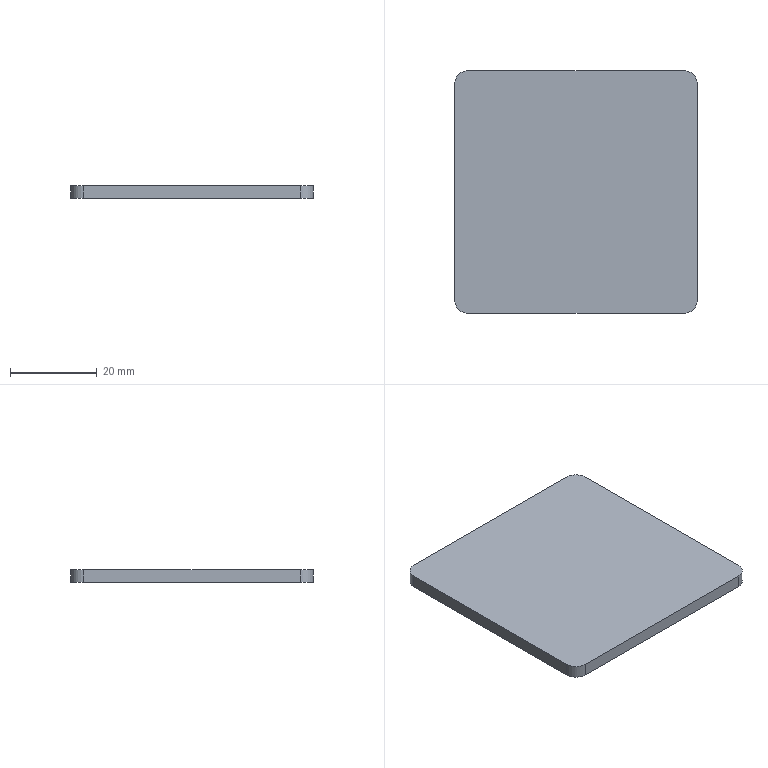Part | STEP file | 750038152 | 1 solid | 10 faces | box 56 x 56 x 3 mm | volume 9385 mm3 | plane 6 | cylinder 4 | commonest cylinder face diameters 6 x4
STEP:
#1=CARTESIAN_POINT('',(28.,25.,3.));
#2=VERTEX_POINT('',#1);
#3=CARTESIAN_POINT('',(25.,28.,3.));
#4=VERTEX_POINT('',#3);
#5=CARTESIAN_POINT('',(25.,25.,3.));
#6=DIRECTION('',(0.,0.,1.));
#7=DIRECTION('',(-1.,0.,0.));
#8=AXIS2_PLACEMENT_3D('',#5,#6,#7);
#9=CIRCLE('',#8,3.);
#10=EDGE_CURVE('',#2,#4,#9,.T.);
#11=ORIENTED_EDGE('',*,*,#10,.T.);
#12=CARTESIAN_POINT('',(-25.,28.,3.));
#13=VERTEX_POINT('',#12);
#14=CARTESIAN_POINT('',(-25.,28.,3.));
#15=DIRECTION('',(-1.,0.,0.));
#16=VECTOR('',#15,1000.);
#17=LINE('',#14,#16);
#18=EDGE_CURVE('',#4,#13,#17,.T.);
#19=ORIENTED_EDGE('',*,*,#18,.T.);
#20=CARTESIAN_POINT('',(-28.,25.,3.));
#21=VERTEX_POINT('',#20);
#22=CARTESIAN_POINT('',(-25.,25.,3.));
#23=DIRECTION('',(0.,0.,1.));
#24=DIRECTION('',(-1.,0.,0.));
#25=AXIS2_PLACEMENT_3D('',#22,#23,#24);
#26=CIRCLE('',#25,3.);
#27=EDGE_CURVE('',#13,#21,#26,.T.);
#28=ORIENTED_EDGE('',*,*,#27,.T.);
#29=CARTESIAN_POINT('',(-28.,-25.,3.));
#30=VERTEX_POINT('',#29);
#31=CARTESIAN_POINT('',(-28.,25.,3.));
#32=DIRECTION('',(0.,-1.,0.));
#33=VECTOR('',#32,1000.);
#34=LINE('',#31,#33);
#35=EDGE_CURVE('',#21,#30,#34,.T.);
#36=ORIENTED_EDGE('',*,*,#35,.T.);
#37=CARTESIAN_POINT('',(-25.,-28.,3.));
#38=VERTEX_POINT('',#37);
#39=CARTESIAN_POINT('',(-25.,-25.,3.));
#40=DIRECTION('',(0.,0.,1.));
#41=DIRECTION('',(-1.,0.,0.));
#42=AXIS2_PLACEMENT_3D('',#39,#40,#41);
#43=CIRCLE('',#42,3.);
#44=EDGE_CURVE('',#30,#38,#43,.T.);
#45=ORIENTED_EDGE('',*,*,#44,.T.);
#46=CARTESIAN_POINT('',(25.,-28.,3.));
#47=VERTEX_POINT('',#46);
#48=CARTESIAN_POINT('',(-25.,-28.,3.));
#49=DIRECTION('',(1.,0.,0.));
#50=VECTOR('',#49,1000.);
#51=LINE('',#48,#50);
#52=EDGE_CURVE('',#38,#47,#51,.T.);
#53=ORIENTED_EDGE('',*,*,#52,.T.);
#54=CARTESIAN_POINT('',(28.,-25.,3.));
#55=VERTEX_POINT('',#54);
#56=CARTESIAN_POINT('',(25.,-25.,3.));
#57=DIRECTION('',(0.,0.,1.));
#58=DIRECTION('',(-1.,0.,0.));
#59=AXIS2_PLACEMENT_3D('',#56,#57,#58);
#60=CIRCLE('',#59,3.);
#61=EDGE_CURVE('',#47,#55,#60,.T.);
#62=ORIENTED_EDGE('',*,*,#61,.T.);
#63=CARTESIAN_POINT('',(28.,25.,3.));
#64=DIRECTION('',(0.,1.,0.));
#65=VECTOR('',#64,1000.);
#66=LINE('',#63,#65);
#67=EDGE_CURVE('',#55,#2,#66,.T.);
#68=ORIENTED_EDGE('',*,*,#67,.T.);
#69=EDGE_LOOP('',(#11,#19,#28,#36,#45,#53,#62,#68));
#70=FACE_OUTER_BOUND('',#69,.T.);
#71=CARTESIAN_POINT('',(-25.,25.,3.));
#72=DIRECTION('',(0.,0.,1.));
#73=DIRECTION('',(1.,0.,0.));
#74=AXIS2_PLACEMENT_3D('',#71,#72,#73);
#75=PLANE('',#74);
#76=ADVANCED_FACE('',(#70),#75,.T.);
#77=CARTESIAN_POINT('',(-25.,28.,0.));
#78=VERTEX_POINT('',#77);
#79=CARTESIAN_POINT('',(-25.,28.,3.));
#80=DIRECTION('',(0.,0.,-1.));
#81=VECTOR('',#80,1000.);
#82=LINE('',#79,#81);
#83=EDGE_CURVE('',#13,#78,#82,.T.);
#84=ORIENTED_EDGE('',*,*,#83,.F.);
#85=ORIENTED_EDGE('',*,*,#18,.F.);
#86=CARTESIAN_POINT('',(25.,28.,0.));
#87=VERTEX_POINT('',#86);
#88=CARTESIAN_POINT('',(25.,28.,3.));
#89=DIRECTION('',(0.,0.,1.));
#90=VECTOR('',#89,1000.);
#91=LINE('',#88,#90);
#92=EDGE_CURVE('',#87,#4,#91,.T.);
#93=ORIENTED_EDGE('',*,*,#92,.F.);
#94=CARTESIAN_POINT('',(25.,28.,0.));
#95=DIRECTION('',(1.,0.,0.));
#96=VECTOR('',#95,1000.);
#97=LINE('',#94,#96);
#98=EDGE_CURVE('',#78,#87,#97,.T.);
#99=ORIENTED_EDGE('',*,*,#98,.F.);
#100=EDGE_LOOP('',(#84,#85,#93,#99));
#101=FACE_OUTER_BOUND('',#100,.T.);
#102=CARTESIAN_POINT('',(25.,28.,3.));
#103=DIRECTION('',(0.,-1.,0.));
#104=DIRECTION('',(0.,0.,-1.));
#105=AXIS2_PLACEMENT_3D('',#102,#103,#104);
#106=PLANE('',#105);
#107=ADVANCED_FACE('',(#101),#106,.F.);
#108=ORIENTED_EDGE('',*,*,#10,.F.);
#109=CARTESIAN_POINT('',(28.,25.,0.));
#110=VERTEX_POINT('',#109);
#111=CARTESIAN_POINT('',(28.,25.,3.));
#112=DIRECTION('',(0.,0.,-1.));
#113=VECTOR('',#112,1000.);
#114=LINE('',#111,#113);
#115=EDGE_CURVE('',#2,#110,#114,.T.);
#116=ORIENTED_EDGE('',*,*,#115,.T.);
#117=CARTESIAN_POINT('',(25.,25.,0.));
#118=DIRECTION('',(0.,0.,1.));
#119=DIRECTION('',(-1.,0.,0.));
#120=AXIS2_PLACEMENT_3D('',#117,#118,#119);
#121=CIRCLE('',#120,3.);
#122=EDGE_CURVE('',#110,#87,#121,.T.);
#123=ORIENTED_EDGE('',*,*,#122,.T.);
#124=ORIENTED_EDGE('',*,*,#92,.T.);
#125=EDGE_LOOP('',(#108,#116,#123,#124));
#126=FACE_OUTER_BOUND('',#125,.T.);
#127=CARTESIAN_POINT('',(25.,25.,3.));
#128=DIRECTION('',(0.,0.,-1.));
#129=DIRECTION('',(-1.,0.,0.));
#130=AXIS2_PLACEMENT_3D('',#127,#128,#129);
#131=CYLINDRICAL_SURFACE('',#130,3.);
#132=ADVANCED_FACE('',(#126),#131,.T.);
#133=ORIENTED_EDGE('',*,*,#115,.F.);
#134=ORIENTED_EDGE('',*,*,#67,.F.);
#135=CARTESIAN_POINT('',(28.,-25.,0.));
#136=VERTEX_POINT('',#135);
#137=CARTESIAN_POINT('',(28.,-25.,3.));
#138=DIRECTION('',(0.,0.,1.));
#139=VECTOR('',#138,1000.);
#140=LINE('',#137,#139);
#141=EDGE_CURVE('',#136,#55,#140,.T.);
#142=ORIENTED_EDGE('',*,*,#141,.F.);
#143=CARTESIAN_POINT('',(28.,-25.,0.));
#144=DIRECTION('',(0.,-1.,0.));
#145=VECTOR('',#144,1000.);
#146=LINE('',#143,#145);
#147=EDGE_CURVE('',#110,#136,#146,.T.);
#148=ORIENTED_EDGE('',*,*,#147,.F.);
#149=EDGE_LOOP('',(#133,#134,#142,#148));
#150=FACE_OUTER_BOUND('',#149,.T.);
#151=CARTESIAN_POINT('',(28.,-25.,3.));
#152=DIRECTION('',(-1.,0.,0.));
#153=DIRECTION('',(0.,-1.,0.));
#154=AXIS2_PLACEMENT_3D('',#151,#152,#153);
#155=PLANE('',#154);
#156=ADVANCED_FACE('',(#150),#155,.F.);
#157=ORIENTED_EDGE('',*,*,#61,.F.);
#158=CARTESIAN_POINT('',(25.,-28.,0.));
#159=VERTEX_POINT('',#158);
#160=CARTESIAN_POINT('',(25.,-28.,3.));
#161=DIRECTION('',(0.,0.,-1.));
#162=VECTOR('',#161,1000.);
#163=LINE('',#160,#162);
#164=EDGE_CURVE('',#47,#159,#163,.T.);
#165=ORIENTED_EDGE('',*,*,#164,.T.);
#166=CARTESIAN_POINT('',(25.,-25.,0.));
#167=DIRECTION('',(0.,0.,1.));
#168=DIRECTION('',(-1.,0.,0.));
#169=AXIS2_PLACEMENT_3D('',#166,#167,#168);
#170=CIRCLE('',#169,3.);
#171=EDGE_CURVE('',#159,#136,#170,.T.);
#172=ORIENTED_EDGE('',*,*,#171,.T.);
#173=ORIENTED_EDGE('',*,*,#141,.T.);
#174=EDGE_LOOP('',(#157,#165,#172,#173));
#175=FACE_OUTER_BOUND('',#174,.T.);
#176=CARTESIAN_POINT('',(25.,-25.,3.));
#177=DIRECTION('',(0.,0.,-1.));
#178=DIRECTION('',(-1.,0.,0.));
#179=AXIS2_PLACEMENT_3D('',#176,#177,#178);
#180=CYLINDRICAL_SURFACE('',#179,3.);
#181=ADVANCED_FACE('',(#175),#180,.T.);
#182=ORIENTED_EDGE('',*,*,#164,.F.);
#183=ORIENTED_EDGE('',*,*,#52,.F.);
#184=CARTESIAN_POINT('',(-25.,-28.,0.));
#185=VERTEX_POINT('',#184);
#186=CARTESIAN_POINT('',(-25.,-28.,3.));
#187=DIRECTION('',(0.,0.,1.));
#188=VECTOR('',#187,1000.);
#189=LINE('',#186,#188);
#190=EDGE_CURVE('',#185,#38,#189,.T.);
#191=ORIENTED_EDGE('',*,*,#190,.F.);
#192=CARTESIAN_POINT('',(-25.,-28.,0.));
#193=DIRECTION('',(-1.,0.,0.));
#194=VECTOR('',#193,1000.);
#195=LINE('',#192,#194);
#196=EDGE_CURVE('',#159,#185,#195,.T.);
#197=ORIENTED_EDGE('',*,*,#196,.F.);
#198=EDGE_LOOP('',(#182,#183,#191,#197));
#199=FACE_OUTER_BOUND('',#198,.T.);
#200=CARTESIAN_POINT('',(-25.,-28.,3.));
#201=DIRECTION('',(0.,1.,0.));
#202=DIRECTION('',(0.,0.,1.));
#203=AXIS2_PLACEMENT_3D('',#200,#201,#202);
#204=PLANE('',#203);
#205=ADVANCED_FACE('',(#199),#204,.F.);
#206=ORIENTED_EDGE('',*,*,#44,.F.);
#207=CARTESIAN_POINT('',(-28.,-25.,0.));
#208=VERTEX_POINT('',#207);
#209=CARTESIAN_POINT('',(-28.,-25.,3.));
#210=DIRECTION('',(0.,0.,-1.));
#211=VECTOR('',#210,1000.);
#212=LINE('',#209,#211);
#213=EDGE_CURVE('',#30,#208,#212,.T.);
#214=ORIENTED_EDGE('',*,*,#213,.T.);
#215=CARTESIAN_POINT('',(-25.,-25.,0.));
#216=DIRECTION('',(0.,0.,1.));
#217=DIRECTION('',(-1.,0.,0.));
#218=AXIS2_PLACEMENT_3D('',#215,#216,#217);
#219=CIRCLE('',#218,3.);
#220=EDGE_CURVE('',#208,#185,#219,.T.);
#221=ORIENTED_EDGE('',*,*,#220,.T.);
#222=ORIENTED_EDGE('',*,*,#190,.T.);
#223=EDGE_LOOP('',(#206,#214,#221,#222));
#224=FACE_OUTER_BOUND('',#223,.T.);
#225=CARTESIAN_POINT('',(-25.,-25.,3.));
#226=DIRECTION('',(0.,0.,-1.));
#227=DIRECTION('',(-1.,0.,0.));
#228=AXIS2_PLACEMENT_3D('',#225,#226,#227);
#229=CYLINDRICAL_SURFACE('',#228,3.);
#230=ADVANCED_FACE('',(#224),#229,.T.);
#231=ORIENTED_EDGE('',*,*,#213,.F.);
#232=ORIENTED_EDGE('',*,*,#35,.F.);
#233=CARTESIAN_POINT('',(-28.,25.,0.));
#234=VERTEX_POINT('',#233);
#235=CARTESIAN_POINT('',(-28.,25.,3.));
#236=DIRECTION('',(0.,0.,1.));
#237=VECTOR('',#236,1000.);
#238=LINE('',#235,#237);
#239=EDGE_CURVE('',#234,#21,#238,.T.);
#240=ORIENTED_EDGE('',*,*,#239,.F.);
#241=CARTESIAN_POINT('',(-28.,25.,0.));
#242=DIRECTION('',(0.,1.,0.));
#243=VECTOR('',#242,1000.);
#244=LINE('',#241,#243);
#245=EDGE_CURVE('',#208,#234,#244,.T.);
#246=ORIENTED_EDGE('',*,*,#245,.F.);
#247=EDGE_LOOP('',(#231,#232,#240,#246));
#248=FACE_OUTER_BOUND('',#247,.T.);
#249=CARTESIAN_POINT('',(-28.,25.,3.));
#250=DIRECTION('',(1.,0.,0.));
#251=DIRECTION('',(0.,1.,0.));
#252=AXIS2_PLACEMENT_3D('',#249,#250,#251);
#253=PLANE('',#252);
#254=ADVANCED_FACE('',(#248),#253,.F.);
#255=ORIENTED_EDGE('',*,*,#27,.F.);
#256=ORIENTED_EDGE('',*,*,#83,.T.);
#257=CARTESIAN_POINT('',(-25.,25.,0.));
#258=DIRECTION('',(0.,0.,1.));
#259=DIRECTION('',(-1.,0.,0.));
#260=AXIS2_PLACEMENT_3D('',#257,#258,#259);
#261=CIRCLE('',#260,3.);
#262=EDGE_CURVE('',#78,#234,#261,.T.);
#263=ORIENTED_EDGE('',*,*,#262,.T.);
#264=ORIENTED_EDGE('',*,*,#239,.T.);
#265=EDGE_LOOP('',(#255,#256,#263,#264));
#266=FACE_OUTER_BOUND('',#265,.T.);
#267=CARTESIAN_POINT('',(-25.,25.,3.));
#268=DIRECTION('',(0.,0.,-1.));
#269=DIRECTION('',(-1.,0.,0.));
#270=AXIS2_PLACEMENT_3D('',#267,#268,#269);
#271=CYLINDRICAL_SURFACE('',#270,3.);
#272=ADVANCED_FACE('',(#266),#271,.T.);
#273=ORIENTED_EDGE('',*,*,#98,.T.);
#274=ORIENTED_EDGE('',*,*,#122,.F.);
#275=ORIENTED_EDGE('',*,*,#147,.T.);
#276=ORIENTED_EDGE('',*,*,#171,.F.);
#277=ORIENTED_EDGE('',*,*,#196,.T.);
#278=ORIENTED_EDGE('',*,*,#220,.F.);
#279=ORIENTED_EDGE('',*,*,#245,.T.);
#280=ORIENTED_EDGE('',*,*,#262,.F.);
#281=EDGE_LOOP('',(#273,#274,#275,#276,#277,#278,#279,#280));
#282=FACE_OUTER_BOUND('',#281,.T.);
#283=CARTESIAN_POINT('',(-25.,25.,0.));
#284=DIRECTION('',(0.,0.,1.));
#285=DIRECTION('',(1.,0.,0.));
#286=AXIS2_PLACEMENT_3D('',#283,#284,#285);
#287=PLANE('',#286);
#288=ADVANCED_FACE('',(#282),#287,.F.);
#289=CLOSED_SHELL('',(#76,#107,#132,#156,#181,#205,#230,#254,#272,#288));
#290=MANIFOLD_SOLID_BREP('',#289);
#291=CARTESIAN_POINT('',(0.,0.,0.));
#292=DIRECTION('',(0.,0.,1.));
#293=DIRECTION('',(1.,0.,0.));
#294=AXIS2_PLACEMENT_3D('',#291,#292,#293);
#295=(LENGTH_UNIT()NAMED_UNIT(*)SI_UNIT(.MILLI.,.METRE.));
#296=UNCERTAINTY_MEASURE_WITH_UNIT(LENGTH_MEASURE(0.00001),#295,'','');
#297=(NAMED_UNIT(*)PLANE_ANGLE_UNIT()SI_UNIT($,.RADIAN.));
#298=(NAMED_UNIT(*)SI_UNIT($,.STERADIAN.)SOLID_ANGLE_UNIT());
#299=(GEOMETRIC_REPRESENTATION_CONTEXT(3)GLOBAL_UNCERTAINTY_ASSIGNED_CONTEXT((#296))GLOBAL_UNIT_ASSIGNED_CONTEXT((#295,#297,#298))REPRESENTATION_CONTEXT('',''));
#300=ADVANCED_BREP_SHAPE_REPRESENTATION('',(#290,#294),#299);